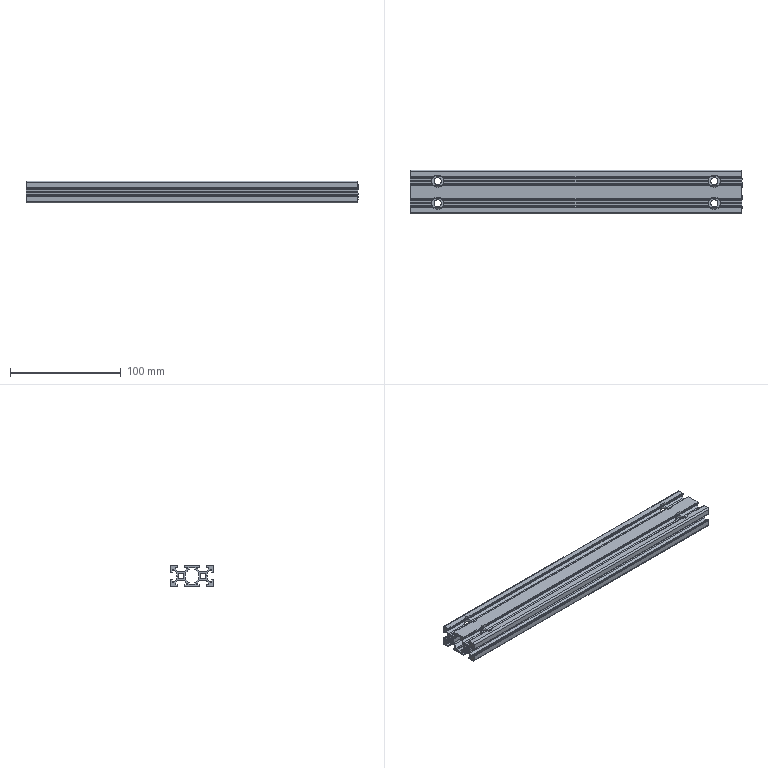Part | STEP file | PN_0001_aluminium profile_default_machined_ | 1 solid | 486 faces | box 300 x 39.479 x 19.74 mm | volume 83778 mm3 | plane 254 | cylinder 232 | commonest cylinder face diameters 0.592 x108 1.123 x33 4.935 x30 3.948 x28 6.6 x14 11 x12